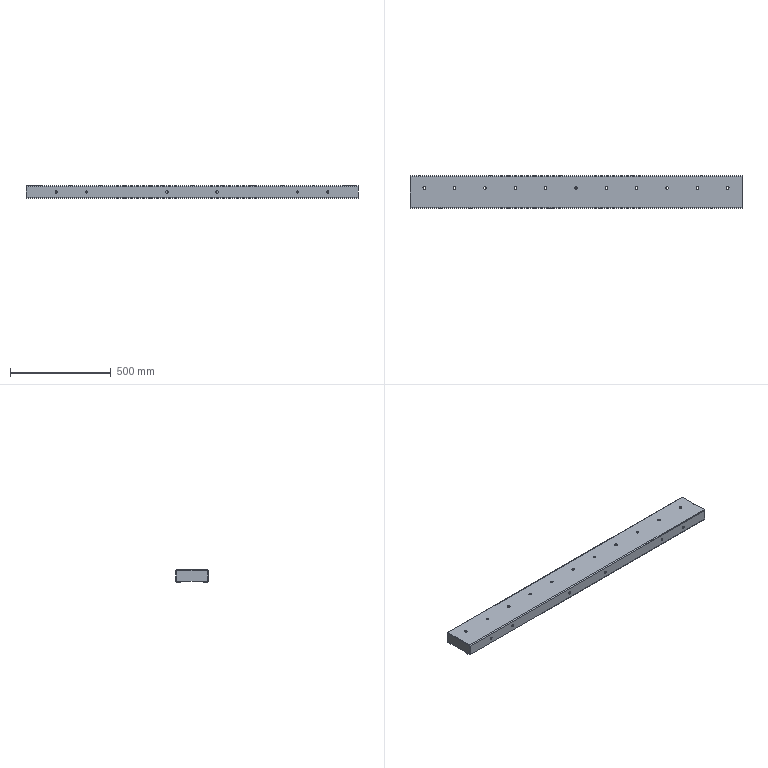Part | STEP file | 3 solids | 90 faces | box 1650 x 160 x 60 mm | volume 2114890 mm3 | cylinder 56 | plane 34 | commonest cylinder face diameters 13 x26 7 x10 11 x8 0.6 x4 1.5 x4 8.6 x4